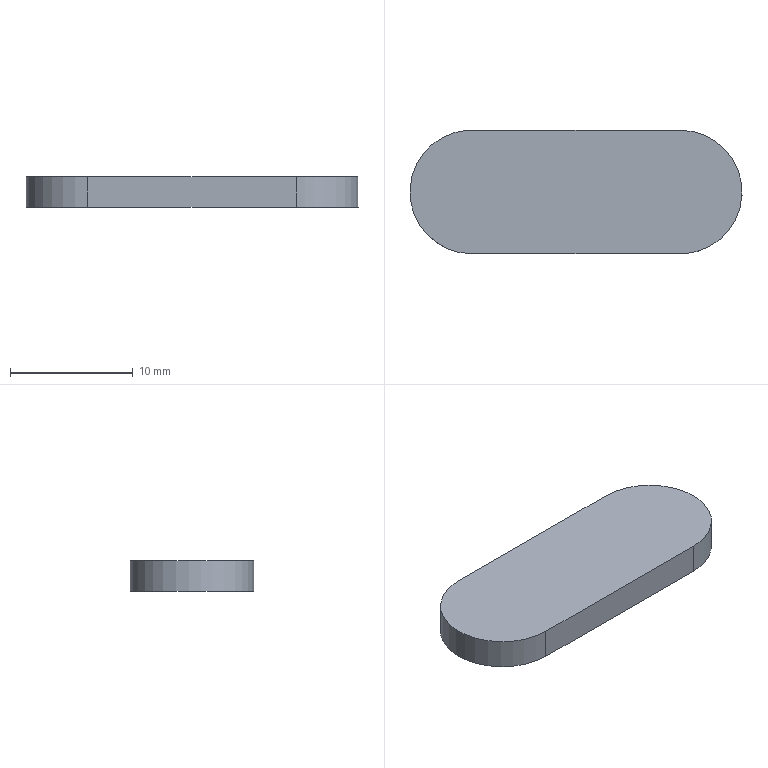Part | STEP file | lll_id414_x_t | 1 solid | 6 faces | box 27.07 x 10.07 x 2.5 mm | volume 626.823 mm3 | plane 4 | spline 2
STEP:
#1=CARTESIAN_POINT('',(3411.,62.035,2.5));
#2=VERTEX_POINT('',#1);
#3=CARTESIAN_POINT('',(3428.,62.035,2.5));
#4=VERTEX_POINT('',#3);
#5=CARTESIAN_POINT('',(3433.,62.035,2.5));
#6=DIRECTION('',(1.,0.,0.000000008));
#7=VECTOR('',#6,1.);
#8=LINE('',#5,#7);
#9=EDGE_CURVE('',#2,#4,#8,.T.);
#10=ORIENTED_EDGE('',*,*,#9,.T.);
#11=CARTESIAN_POINT('',(3428.,62.035,0.00001778));
#12=VERTEX_POINT('',#11);
#13=CARTESIAN_POINT('',(3428.,62.035,0.00001778));
#14=DIRECTION('',(-0.000000008,0.,1.));
#15=VECTOR('',#14,1.);
#16=LINE('',#13,#15);
#17=EDGE_CURVE('',#12,#4,#16,.T.);
#18=ORIENTED_EDGE('',*,*,#17,.F.);
#19=CARTESIAN_POINT('',(3411.,62.035,0.00001765));
#20=VERTEX_POINT('',#19);
#21=CARTESIAN_POINT('',(3433.,62.035,0.00001781));
#22=DIRECTION('',(1.,0.,0.000000008));
#23=VECTOR('',#22,1.);
#24=LINE('',#21,#23);
#25=EDGE_CURVE('',#20,#12,#24,.T.);
#26=ORIENTED_EDGE('',*,*,#25,.F.);
#27=CARTESIAN_POINT('',(3411.,62.035,0.00001765));
#28=DIRECTION('',(-0.000000008,0.,1.));
#29=VECTOR('',#28,1.);
#30=LINE('',#27,#29);
#31=EDGE_CURVE('',#20,#2,#30,.T.);
#32=ORIENTED_EDGE('',*,*,#31,.T.);
#33=EDGE_LOOP('',(#10,#18,#26,#32));
#34=FACE_OUTER_BOUND('',#33,.T.);
#35=CARTESIAN_POINT('',(3411.,62.035,0.00001765));
#36=DIRECTION('',(0.,-1.,0.));
#37=DIRECTION('',(-0.000000008,0.,1.));
#38=AXIS2_PLACEMENT_3D('',#35,#36,#37);
#39=PLANE('',#38);
#40=ADVANCED_FACE('',(#34),#39,.F.);
#41=CARTESIAN_POINT('',(3428.,51.965,2.5));
#42=VERTEX_POINT('',#41);
#43=CARTESIAN_POINT('',(3428.,62.035,2.5));
#44=CARTESIAN_POINT('',(3429.318,62.035,2.5));
#45=CARTESIAN_POINT('',(3430.628,61.493,2.5));
#46=CARTESIAN_POINT('',(3432.493,59.628,2.5));
#47=CARTESIAN_POINT('',(3433.035,58.319,2.5));
#48=CARTESIAN_POINT('',(3433.035,55.682,2.5));
#49=CARTESIAN_POINT('',(3432.493,54.372,2.5));
#50=CARTESIAN_POINT('',(3430.628,52.508,2.5));
#51=CARTESIAN_POINT('',(3429.318,51.965,2.5));
#52=CARTESIAN_POINT('',(3428.,51.965,2.5));
#53=B_SPLINE_CURVE_WITH_KNOTS('',3,(#43,#44,#45,#46,#47,#48,#49,#50,#51,#52),.UNSPECIFIED.,.F.,.F.,(4,2,2,2,4),(0.,0.25,0.5,0.75,1.),.UNSPECIFIED.);
#54=EDGE_CURVE('',#4,#42,#53,.T.);
#55=ORIENTED_EDGE('',*,*,#54,.T.);
#56=CARTESIAN_POINT('',(3428.,51.965,0.00001778));
#57=VERTEX_POINT('',#56);
#58=CARTESIAN_POINT('',(3428.,51.965,0.00001778));
#59=DIRECTION('',(-0.000000008,0.,1.));
#60=VECTOR('',#59,1.);
#61=LINE('',#58,#60);
#62=EDGE_CURVE('',#57,#42,#61,.T.);
#63=ORIENTED_EDGE('',*,*,#62,.F.);
#64=CARTESIAN_POINT('',(3428.,62.035,0.00001778));
#65=CARTESIAN_POINT('',(3429.318,62.035,0.00001779));
#66=CARTESIAN_POINT('',(3430.628,61.493,0.0000178));
#67=CARTESIAN_POINT('',(3432.493,59.628,0.00001781));
#68=CARTESIAN_POINT('',(3433.035,58.319,0.00001781));
#69=CARTESIAN_POINT('',(3433.035,55.682,0.00001781));
#70=CARTESIAN_POINT('',(3432.493,54.372,0.00001781));
#71=CARTESIAN_POINT('',(3430.628,52.508,0.0000178));
#72=CARTESIAN_POINT('',(3429.318,51.965,0.00001779));
#73=CARTESIAN_POINT('',(3428.,51.965,0.00001778));
#74=B_SPLINE_CURVE_WITH_KNOTS('',3,(#64,#65,#66,#67,#68,#69,#70,#71,#72,#73),.UNSPECIFIED.,.F.,.F.,(4,2,2,2,4),(0.,0.25,0.5,0.75,1.),.UNSPECIFIED.);
#75=EDGE_CURVE('',#12,#57,#74,.T.);
#76=ORIENTED_EDGE('',*,*,#75,.F.);
#77=ORIENTED_EDGE('',*,*,#17,.T.);
#78=EDGE_LOOP('',(#55,#63,#76,#77));
#79=FACE_OUTER_BOUND('',#78,.T.);
#80=CARTESIAN_POINT('',(3428.,51.965,0.00001778));
#81=CARTESIAN_POINT('',(3428.,51.965,2.5));
#82=CARTESIAN_POINT('',(3429.318,51.965,0.00001779));
#83=CARTESIAN_POINT('',(3429.318,51.965,2.5));
#84=CARTESIAN_POINT('',(3430.628,52.508,0.0000178));
#85=CARTESIAN_POINT('',(3430.628,52.508,2.5));
#86=CARTESIAN_POINT('',(3432.493,54.372,0.00001781));
#87=CARTESIAN_POINT('',(3432.493,54.372,2.5));
#88=CARTESIAN_POINT('',(3433.035,55.682,0.00001781));
#89=CARTESIAN_POINT('',(3433.035,55.682,2.5));
#90=CARTESIAN_POINT('',(3433.035,58.319,0.00001781));
#91=CARTESIAN_POINT('',(3433.035,58.319,2.5));
#92=CARTESIAN_POINT('',(3432.493,59.628,0.00001781));
#93=CARTESIAN_POINT('',(3432.493,59.628,2.5));
#94=CARTESIAN_POINT('',(3430.628,61.493,0.0000178));
#95=CARTESIAN_POINT('',(3430.628,61.493,2.5));
#96=CARTESIAN_POINT('',(3429.318,62.035,0.00001779));
#97=CARTESIAN_POINT('',(3429.318,62.035,2.5));
#98=CARTESIAN_POINT('',(3428.,62.035,0.00001778));
#99=CARTESIAN_POINT('',(3428.,62.035,2.5));
#100=B_SPLINE_SURFACE_WITH_KNOTS('',3,1,((#80,#81),(#82,#83),(#84,#85),(#86,#87),(#88,#89),(#90,#91),(#92,#93),(#94,#95),(#96,#97),(#98,#99)),.UNSPECIFIED.,.F.,.F.,.F.,(4,2,2,2,4),(2,2),(0.,0.25,0.5,0.75,1.),(0.,1.),.UNSPECIFIED.);
#101=ADVANCED_FACE('',(#79),#100,.T.);
#102=CARTESIAN_POINT('',(3411.,51.965,2.5));
#103=VERTEX_POINT('',#102);
#104=CARTESIAN_POINT('',(3433.,51.965,2.5));
#105=DIRECTION('',(-1.,0.,-0.000000008));
#106=VECTOR('',#105,1.);
#107=LINE('',#104,#106);
#108=EDGE_CURVE('',#42,#103,#107,.T.);
#109=ORIENTED_EDGE('',*,*,#108,.T.);
#110=CARTESIAN_POINT('',(3411.,51.965,0.00001765));
#111=VERTEX_POINT('',#110);
#112=CARTESIAN_POINT('',(3411.,51.965,0.00001765));
#113=DIRECTION('',(-0.000000008,0.,1.));
#114=VECTOR('',#113,1.);
#115=LINE('',#112,#114);
#116=EDGE_CURVE('',#111,#103,#115,.T.);
#117=ORIENTED_EDGE('',*,*,#116,.F.);
#118=CARTESIAN_POINT('',(3433.,51.965,0.00001781));
#119=DIRECTION('',(-1.,0.,-0.000000008));
#120=VECTOR('',#119,1.);
#121=LINE('',#118,#120);
#122=EDGE_CURVE('',#57,#111,#121,.T.);
#123=ORIENTED_EDGE('',*,*,#122,.F.);
#124=ORIENTED_EDGE('',*,*,#62,.T.);
#125=EDGE_LOOP('',(#109,#117,#123,#124));
#126=FACE_OUTER_BOUND('',#125,.T.);
#127=CARTESIAN_POINT('',(3428.,51.965,0.00001778));
#128=DIRECTION('',(0.,1.,0.));
#129=DIRECTION('',(0.000000008,0.,-1.));
#130=AXIS2_PLACEMENT_3D('',#127,#128,#129);
#131=PLANE('',#130);
#132=ADVANCED_FACE('',(#126),#131,.F.);
#133=CARTESIAN_POINT('',(3411.,51.965,2.5));
#134=CARTESIAN_POINT('',(3409.691,51.965,2.5));
#135=CARTESIAN_POINT('',(3408.372,52.508,2.5));
#136=CARTESIAN_POINT('',(3406.507,54.372,2.5));
#137=CARTESIAN_POINT('',(3405.965,55.682,2.5));
#138=CARTESIAN_POINT('',(3405.965,58.319,2.5));
#139=CARTESIAN_POINT('',(3406.507,59.628,2.5));
#140=CARTESIAN_POINT('',(3408.372,61.493,2.5));
#141=CARTESIAN_POINT('',(3409.682,62.035,2.5));
#142=CARTESIAN_POINT('',(3411.,62.035,2.5));
#143=B_SPLINE_CURVE_WITH_KNOTS('',3,(#133,#134,#135,#136,#137,#138,#139,#140,#141,#142),.UNSPECIFIED.,.F.,.F.,(4,2,2,2,4),(0.,0.25,0.5,0.75,1.),.UNSPECIFIED.);
#144=EDGE_CURVE('',#103,#2,#143,.T.);
#145=ORIENTED_EDGE('',*,*,#144,.T.);
#146=ORIENTED_EDGE('',*,*,#31,.F.);
#147=CARTESIAN_POINT('',(3411.,51.965,0.00001765));
#148=CARTESIAN_POINT('',(3409.691,51.965,0.00001764));
#149=CARTESIAN_POINT('',(3408.372,52.508,0.00001763));
#150=CARTESIAN_POINT('',(3406.507,54.372,0.00001761));
#151=CARTESIAN_POINT('',(3405.965,55.682,0.00001761));
#152=CARTESIAN_POINT('',(3405.965,58.319,0.00001761));
#153=CARTESIAN_POINT('',(3406.507,59.628,0.00001761));
#154=CARTESIAN_POINT('',(3408.372,61.493,0.00001763));
#155=CARTESIAN_POINT('',(3409.682,62.035,0.00001764));
#156=CARTESIAN_POINT('',(3411.,62.035,0.00001765));
#157=B_SPLINE_CURVE_WITH_KNOTS('',3,(#147,#148,#149,#150,#151,#152,#153,#154,#155,#156),.UNSPECIFIED.,.F.,.F.,(4,2,2,2,4),(0.,0.25,0.5,0.75,1.),.UNSPECIFIED.);
#158=EDGE_CURVE('',#111,#20,#157,.T.);
#159=ORIENTED_EDGE('',*,*,#158,.F.);
#160=ORIENTED_EDGE('',*,*,#116,.T.);
#161=EDGE_LOOP('',(#145,#146,#159,#160));
#162=FACE_OUTER_BOUND('',#161,.T.);
#163=CARTESIAN_POINT('',(3411.,62.035,0.00001765));
#164=CARTESIAN_POINT('',(3411.,62.035,2.5));
#165=CARTESIAN_POINT('',(3409.682,62.035,0.00001764));
#166=CARTESIAN_POINT('',(3409.682,62.035,2.5));
#167=CARTESIAN_POINT('',(3408.372,61.493,0.00001763));
#168=CARTESIAN_POINT('',(3408.372,61.493,2.5));
#169=CARTESIAN_POINT('',(3406.507,59.628,0.00001761));
#170=CARTESIAN_POINT('',(3406.507,59.628,2.5));
#171=CARTESIAN_POINT('',(3405.965,58.319,0.00001761));
#172=CARTESIAN_POINT('',(3405.965,58.319,2.5));
#173=CARTESIAN_POINT('',(3405.965,55.682,0.00001761));
#174=CARTESIAN_POINT('',(3405.965,55.682,2.5));
#175=CARTESIAN_POINT('',(3406.507,54.372,0.00001761));
#176=CARTESIAN_POINT('',(3406.507,54.372,2.5));
#177=CARTESIAN_POINT('',(3408.372,52.508,0.00001763));
#178=CARTESIAN_POINT('',(3408.372,52.508,2.5));
#179=CARTESIAN_POINT('',(3409.691,51.965,0.00001764));
#180=CARTESIAN_POINT('',(3409.691,51.965,2.5));
#181=CARTESIAN_POINT('',(3411.,51.965,0.00001765));
#182=CARTESIAN_POINT('',(3411.,51.965,2.5));
#183=B_SPLINE_SURFACE_WITH_KNOTS('',3,1,((#163,#164),(#165,#166),(#167,#168),(#169,#170),(#171,#172),(#173,#174),(#175,#176),(#177,#178),(#179,#180),(#181,#182)),.UNSPECIFIED.,.F.,.F.,.F.,(4,2,2,2,4),(2,2),(0.,0.25,0.5,0.75,1.),(0.,1.),.UNSPECIFIED.);
#184=ADVANCED_FACE('',(#162),#183,.T.);
#185=ORIENTED_EDGE('',*,*,#25,.T.);
#186=ORIENTED_EDGE('',*,*,#75,.T.);
#187=ORIENTED_EDGE('',*,*,#122,.T.);
#188=ORIENTED_EDGE('',*,*,#158,.T.);
#189=EDGE_LOOP('',(#185,#186,#187,#188));
#190=FACE_OUTER_BOUND('',#189,.T.);
#191=CARTESIAN_POINT('',(3433.,57.,0.00001781));
#192=DIRECTION('',(-0.000000008,0.,1.));
#193=DIRECTION('',(0.,1.,0.));
#194=AXIS2_PLACEMENT_3D('',#191,#192,#193);
#195=PLANE('',#194);
#196=ADVANCED_FACE('',(#190),#195,.F.);
#197=ORIENTED_EDGE('',*,*,#9,.F.);
#198=ORIENTED_EDGE('',*,*,#144,.F.);
#199=ORIENTED_EDGE('',*,*,#108,.F.);
#200=ORIENTED_EDGE('',*,*,#54,.F.);
#201=EDGE_LOOP('',(#197,#198,#199,#200));
#202=FACE_OUTER_BOUND('',#201,.T.);
#203=CARTESIAN_POINT('',(3433.,57.,2.5));
#204=DIRECTION('',(-0.000000008,0.,1.));
#205=DIRECTION('',(0.,1.,0.));
#206=AXIS2_PLACEMENT_3D('',#203,#204,#205);
#207=PLANE('',#206);
#208=ADVANCED_FACE('',(#202),#207,.T.);
#209=CLOSED_SHELL('',(#40,#101,#132,#184,#196,#208));
#210=MANIFOLD_SOLID_BREP('',#209);
#211=(LENGTH_UNIT()NAMED_UNIT(*)SI_UNIT(.MILLI.,.METRE.));
#212=UNCERTAINTY_MEASURE_WITH_UNIT(LENGTH_MEASURE(0.00002),#211,'','');
#213=(NAMED_UNIT(*)PLANE_ANGLE_UNIT()SI_UNIT($,.RADIAN.));
#214=PLANE_ANGLE_MEASURE_WITH_UNIT(PLANE_ANGLE_MEASURE(0.01745),#213);
#215=DIMENSIONAL_EXPONENTS(0.,0.,0.,0.,0.,0.,0.);
#216=(CONVERSION_BASED_UNIT('DEGREE',#214)NAMED_UNIT(#215)PLANE_ANGLE_UNIT());
#217=(NAMED_UNIT(*)SI_UNIT($,.STERADIAN.)SOLID_ANGLE_UNIT());
#218=(GEOMETRIC_REPRESENTATION_CONTEXT(3)GLOBAL_UNCERTAINTY_ASSIGNED_CONTEXT((#212))GLOBAL_UNIT_ASSIGNED_CONTEXT((#211,#216,#217))REPRESENTATION_CONTEXT('',''));
#219=ADVANCED_BREP_SHAPE_REPRESENTATION('',(#210),#218);